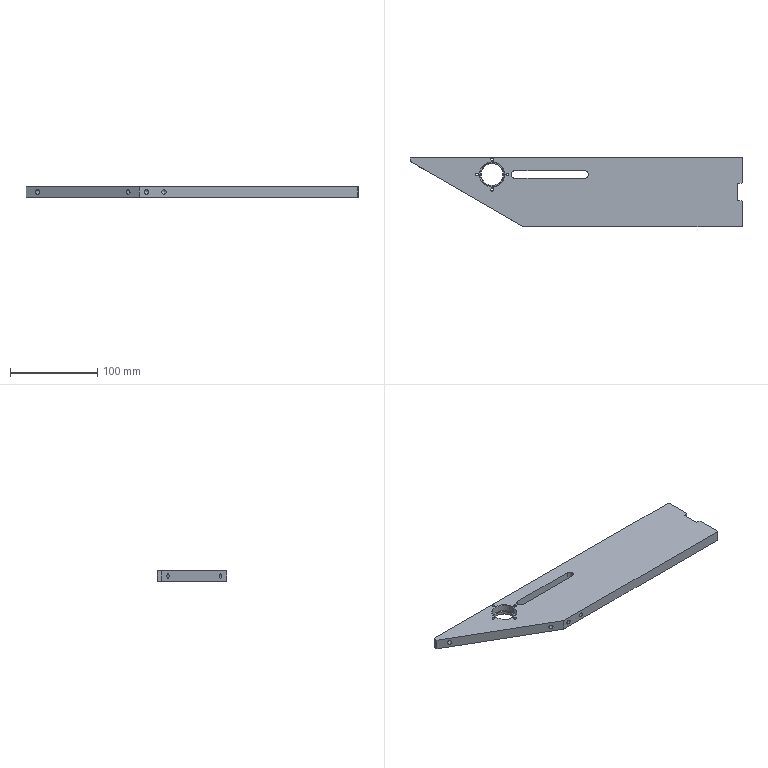Part | NX | 1 solid | 42 faces | box 380 x 80 x 12 mm | volume 287140 mm3 | plane 19 | cylinder 14 | cone 9 | commonest cylinder face diameters 5 x6 3.3 x4 8.5 x2 25 x1 28 x1
STEP:
#1=CARTESIAN_POINT('',(190.,-32.5,-6.));
#2=VERTEX_POINT('',#1);
#3=CARTESIAN_POINT('',(190.,-30.,-6.));
#4=DIRECTION('',(1.,0.,0.));
#5=DIRECTION('',(0.,-1.,0.));
#6=AXIS2_PLACEMENT_3D('',#3,#4,#5);
#7=CIRCLE('',#6,2.5);
#8=EDGE_CURVE('',#2,#2,#7,.T.);
#9=ORIENTED_EDGE('',*,*,#8,.F.);
#10=EDGE_LOOP('',(#9));
#11=FACE_BOUND('',#10,.T.);
#12=CARTESIAN_POINT('',(190.,-11.,-12.));
#13=VERTEX_POINT('',#12);
#14=CARTESIAN_POINT('',(190.,-39.,-12.));
#15=VERTEX_POINT('',#14);
#16=CARTESIAN_POINT('',(190.,40.,-12.));
#17=DIRECTION('',(0.,-1.,0.));
#18=VECTOR('',#17,1000.);
#19=LINE('',#16,#18);
#20=EDGE_CURVE('',#13,#15,#19,.T.);
#21=ORIENTED_EDGE('',*,*,#20,.F.);
#22=CARTESIAN_POINT('',(190.,-11.,0.));
#23=VERTEX_POINT('',#22);
#24=CARTESIAN_POINT('',(190.,-11.,-12.));
#25=DIRECTION('',(0.,0.,1.));
#26=VECTOR('',#25,1000.);
#27=LINE('',#24,#26);
#28=EDGE_CURVE('',#13,#23,#27,.T.);
#29=ORIENTED_EDGE('',*,*,#28,.T.);
#30=CARTESIAN_POINT('',(190.,-39.,0.));
#31=VERTEX_POINT('',#30);
#32=CARTESIAN_POINT('',(190.,40.,0.));
#33=DIRECTION('',(0.,-1.,0.));
#34=VECTOR('',#33,1000.);
#35=LINE('',#32,#34);
#36=EDGE_CURVE('',#23,#31,#35,.T.);
#37=ORIENTED_EDGE('',*,*,#36,.T.);
#38=CARTESIAN_POINT('',(190.,-39.,-12.));
#39=DIRECTION('',(0.,0.,-1.));
#40=VECTOR('',#39,1000.);
#41=LINE('',#38,#40);
#42=EDGE_CURVE('',#31,#15,#41,.T.);
#43=ORIENTED_EDGE('',*,*,#42,.T.);
#44=EDGE_LOOP('',(#21,#29,#37,#43));
#45=FACE_BOUND('',#44,.T.);
#46=CARTESIAN_POINT('',(190.,40.,-12.));
#47=DIRECTION('',(-1.,0.,0.));
#48=DIRECTION('',(0.,1.,0.));
#49=AXIS2_PLACEMENT_3D('',#46,#47,#48);
#50=PLANE('',#49);
#51=ADVANCED_FACE('',(#11,#45),#50,.F.);
#52=CARTESIAN_POINT('',(-96.,32.5,-8.5));
#53=VERTEX_POINT('',#52);
#54=CARTESIAN_POINT('',(-96.,20.,-8.5));
#55=DIRECTION('',(0.,0.,1.));
#56=DIRECTION('',(0.,1.,0.));
#57=AXIS2_PLACEMENT_3D('',#54,#55,#56);
#58=CIRCLE('',#57,12.5);
#59=EDGE_CURVE('',#53,#53,#58,.T.);
#60=ORIENTED_EDGE('',*,*,#59,.T.);
#61=EDGE_LOOP('',(#60));
#62=FACE_BOUND('',#61,.T.);
#63=CARTESIAN_POINT('',(-96.,32.5,-11.5));
#64=VERTEX_POINT('',#63);
#65=CARTESIAN_POINT('',(-96.,20.,-11.5));
#66=DIRECTION('',(0.,0.,1.));
#67=DIRECTION('',(0.,1.,0.));
#68=AXIS2_PLACEMENT_3D('',#65,#66,#67);
#69=CIRCLE('',#68,12.5);
#70=EDGE_CURVE('',#64,#64,#69,.F.);
#71=ORIENTED_EDGE('',*,*,#70,.T.);
#72=EDGE_LOOP('',(#71));
#73=FACE_BOUND('',#72,.T.);
#74=CARTESIAN_POINT('',(-96.,20.,0.));
#75=DIRECTION('',(0.,0.,-1.));
#76=DIRECTION('',(0.,-1.,0.));
#77=AXIS2_PLACEMENT_3D('',#74,#75,#76);
#78=CYLINDRICAL_SURFACE('',#77,12.5);
#79=ADVANCED_FACE('',(#62,#73),#78,.F.);
#80=CARTESIAN_POINT('',(-168.66,40.,-8.3));
#81=VERTEX_POINT('',#80);
#82=CARTESIAN_POINT('',(-168.66,40.,-3.7));
#83=VERTEX_POINT('',#82);
#84=CARTESIAN_POINT('',(-168.66,40.,-8.3));
#85=CARTESIAN_POINT('',(-168.16,40.,-7.644));
#86=CARTESIAN_POINT('',(-167.409,40.,-6.001));
#87=CARTESIAN_POINT('',(-168.153,40.,-4.365));
#88=CARTESIAN_POINT('',(-168.66,40.,-3.7));
#89=B_SPLINE_CURVE_WITH_KNOTS('',3,(#84,#85,#86,#87,#88),.UNSPECIFIED.,.F.,.F.,(4,1,4),(0.001159,0.003632,0.006106),.UNSPECIFIED.);
#90=EDGE_CURVE('',#81,#83,#89,.T.);
#91=ORIENTED_EDGE('',*,*,#90,.T.);
#92=CARTESIAN_POINT('',(-169.793,40.,-6.));
#93=DIRECTION('',(0.,-1.,0.));
#94=DIRECTION('',(-1.,0.,0.));
#95=AXIS2_PLACEMENT_3D('',#92,#93,#94);
#96=ELLIPSE('',#95,2.887,2.5);
#97=EDGE_CURVE('',#83,#81,#96,.T.);
#98=ORIENTED_EDGE('',*,*,#97,.T.);
#99=EDGE_LOOP('',(#91,#98));
#100=FACE_BOUND('',#99,.T.);
#101=CARTESIAN_POINT('',(-189.,40.,-12.));
#102=VERTEX_POINT('',#101);
#103=CARTESIAN_POINT('',(189.,40.,-12.));
#104=VERTEX_POINT('',#103);
#105=CARTESIAN_POINT('',(190.,40.,-12.));
#106=DIRECTION('',(1.,0.,0.));
#107=VECTOR('',#106,1000.);
#108=LINE('',#105,#107);
#109=EDGE_CURVE('',#102,#104,#108,.T.);
#110=ORIENTED_EDGE('',*,*,#109,.F.);
#111=CARTESIAN_POINT('',(-189.,40.,0.));
#112=VERTEX_POINT('',#111);
#113=CARTESIAN_POINT('',(-189.,40.,-12.));
#114=DIRECTION('',(0.,0.,1.));
#115=VECTOR('',#114,1000.);
#116=LINE('',#113,#115);
#117=EDGE_CURVE('',#102,#112,#116,.T.);
#118=ORIENTED_EDGE('',*,*,#117,.T.);
#119=CARTESIAN_POINT('',(189.,40.,0.));
#120=VERTEX_POINT('',#119);
#121=CARTESIAN_POINT('',(190.,40.,0.));
#122=DIRECTION('',(1.,0.,0.));
#123=VECTOR('',#122,1000.);
#124=LINE('',#121,#123);
#125=EDGE_CURVE('',#112,#120,#124,.T.);
#126=ORIENTED_EDGE('',*,*,#125,.T.);
#127=CARTESIAN_POINT('',(189.,40.,-12.));
#128=DIRECTION('',(0.,0.,-1.));
#129=VECTOR('',#128,1000.);
#130=LINE('',#127,#129);
#131=EDGE_CURVE('',#120,#104,#130,.T.);
#132=ORIENTED_EDGE('',*,*,#131,.T.);
#133=EDGE_LOOP('',(#110,#118,#126,#132));
#134=FACE_BOUND('',#133,.T.);
#135=CARTESIAN_POINT('',(190.,40.,-12.));
#136=DIRECTION('',(0.,-1.,0.));
#137=DIRECTION('',(0.,0.,1.));
#138=AXIS2_PLACEMENT_3D('',#135,#136,#137);
#139=PLANE('',#138);
#140=ADVANCED_FACE('',(#100,#134),#139,.F.);
#141=CARTESIAN_POINT('',(190.,27.5,-6.));
#142=VERTEX_POINT('',#141);
#143=CARTESIAN_POINT('',(190.,30.,-6.));
#144=DIRECTION('',(1.,0.,0.));
#145=DIRECTION('',(0.,-1.,0.));
#146=AXIS2_PLACEMENT_3D('',#143,#144,#145);
#147=CIRCLE('',#146,2.5);
#148=EDGE_CURVE('',#142,#142,#147,.T.);
#149=ORIENTED_EDGE('',*,*,#148,.F.);
#150=EDGE_LOOP('',(#149));
#151=FACE_BOUND('',#150,.T.);
#152=CARTESIAN_POINT('',(190.,39.,0.));
#153=VERTEX_POINT('',#152);
#154=CARTESIAN_POINT('',(190.,11.,0.));
#155=VERTEX_POINT('',#154);
#156=CARTESIAN_POINT('',(190.,40.,0.));
#157=DIRECTION('',(0.,-1.,0.));
#158=VECTOR('',#157,1000.);
#159=LINE('',#156,#158);
#160=EDGE_CURVE('',#153,#155,#159,.T.);
#161=ORIENTED_EDGE('',*,*,#160,.T.);
#162=CARTESIAN_POINT('',(190.,11.,-12.));
#163=VERTEX_POINT('',#162);
#164=CARTESIAN_POINT('',(190.,11.,-12.));
#165=DIRECTION('',(0.,0.,-1.));
#166=VECTOR('',#165,1000.);
#167=LINE('',#164,#166);
#168=EDGE_CURVE('',#155,#163,#167,.T.);
#169=ORIENTED_EDGE('',*,*,#168,.T.);
#170=CARTESIAN_POINT('',(190.,39.,-12.));
#171=VERTEX_POINT('',#170);
#172=CARTESIAN_POINT('',(190.,40.,-12.));
#173=DIRECTION('',(0.,-1.,0.));
#174=VECTOR('',#173,1000.);
#175=LINE('',#172,#174);
#176=EDGE_CURVE('',#171,#163,#175,.T.);
#177=ORIENTED_EDGE('',*,*,#176,.F.);
#178=CARTESIAN_POINT('',(190.,39.,-12.));
#179=DIRECTION('',(0.,0.,1.));
#180=VECTOR('',#179,1000.);
#181=LINE('',#178,#180);
#182=EDGE_CURVE('',#171,#153,#181,.T.);
#183=ORIENTED_EDGE('',*,*,#182,.T.);
#184=EDGE_LOOP('',(#161,#169,#177,#183));
#185=FACE_BOUND('',#184,.T.);
#186=CARTESIAN_POINT('',(190.,40.,-12.));
#187=DIRECTION('',(-1.,0.,0.));
#188=DIRECTION('',(0.,1.,0.));
#189=AXIS2_PLACEMENT_3D('',#186,#187,#188);
#190=PLANE('',#189);
#191=ADVANCED_FACE('',(#151,#185),#190,.F.);
#192=CARTESIAN_POINT('',(-52.096,-40.,-3.5));
#193=VERTEX_POINT('',#192);
#194=CARTESIAN_POINT('',(-52.096,-40.,-6.));
#195=DIRECTION('',(0.,-1.,0.));
#196=DIRECTION('',(0.,0.,1.));
#197=AXIS2_PLACEMENT_3D('',#194,#195,#196);
#198=CIRCLE('',#197,2.5);
#199=EDGE_CURVE('',#193,#193,#198,.T.);
#200=ORIENTED_EDGE('',*,*,#199,.F.);
#201=EDGE_LOOP('',(#200));
#202=FACE_BOUND('',#201,.T.);
#203=CARTESIAN_POINT('',(-32.096,-40.,-3.5));
#204=VERTEX_POINT('',#203);
#205=CARTESIAN_POINT('',(-32.096,-40.,-6.));
#206=DIRECTION('',(0.,-1.,0.));
#207=DIRECTION('',(0.,0.,1.));
#208=AXIS2_PLACEMENT_3D('',#205,#206,#207);
#209=CIRCLE('',#208,2.5);
#210=EDGE_CURVE('',#204,#204,#209,.T.);
#211=ORIENTED_EDGE('',*,*,#210,.F.);
#212=EDGE_LOOP('',(#211));
#213=FACE_BOUND('',#212,.T.);
#214=CARTESIAN_POINT('',(189.,-40.,-12.));
#215=VERTEX_POINT('',#214);
#216=CARTESIAN_POINT('',(-60.096,-40.,-12.));
#217=VERTEX_POINT('',#216);
#218=CARTESIAN_POINT('',(190.,-40.,-12.));
#219=DIRECTION('',(-1.,0.,0.));
#220=VECTOR('',#219,1000.);
#221=LINE('',#218,#220);
#222=EDGE_CURVE('',#215,#217,#221,.T.);
#223=ORIENTED_EDGE('',*,*,#222,.F.);
#224=CARTESIAN_POINT('',(189.,-40.,0.));
#225=VERTEX_POINT('',#224);
#226=CARTESIAN_POINT('',(189.,-40.,-12.));
#227=DIRECTION('',(0.,0.,1.));
#228=VECTOR('',#227,1000.);
#229=LINE('',#226,#228);
#230=EDGE_CURVE('',#215,#225,#229,.T.);
#231=ORIENTED_EDGE('',*,*,#230,.T.);
#232=CARTESIAN_POINT('',(-60.096,-40.,0.));
#233=VERTEX_POINT('',#232);
#234=CARTESIAN_POINT('',(190.,-40.,0.));
#235=DIRECTION('',(-1.,0.,0.));
#236=VECTOR('',#235,1000.);
#237=LINE('',#234,#236);
#238=EDGE_CURVE('',#225,#233,#237,.T.);
#239=ORIENTED_EDGE('',*,*,#238,.T.);
#240=CARTESIAN_POINT('',(-60.096,-40.,-12.));
#241=DIRECTION('',(0.,0.,1.));
#242=VECTOR('',#241,1000.);
#243=LINE('',#240,#242);
#244=EDGE_CURVE('',#217,#233,#243,.T.);
#245=ORIENTED_EDGE('',*,*,#244,.F.);
#246=EDGE_LOOP('',(#223,#231,#239,#245));
#247=FACE_BOUND('',#246,.T.);
#248=CARTESIAN_POINT('',(190.,-40.,-12.));
#249=DIRECTION('',(0.,1.,0.));
#250=DIRECTION('',(0.,0.,-1.));
#251=AXIS2_PLACEMENT_3D('',#248,#249,#250);
#252=PLANE('',#251);
#253=ADVANCED_FACE('',(#202,#213,#247),#252,.F.);
#254=CARTESIAN_POINT('',(-179.175,28.75,-6.));
#255=VERTEX_POINT('',#254);
#256=CARTESIAN_POINT('',(-177.01,27.5,-6.));
#257=DIRECTION('',(-0.5,-0.866,0.));
#258=DIRECTION('',(-0.866,0.5,0.));
#259=AXIS2_PLACEMENT_3D('',#256,#257,#258);
#260=CIRCLE('',#259,2.5);
#261=EDGE_CURVE('',#255,#255,#260,.T.);
#262=ORIENTED_EDGE('',*,*,#261,.F.);
#263=EDGE_LOOP('',(#262));
#264=FACE_BOUND('',#263,.T.);
#265=CARTESIAN_POINT('',(-75.252,-31.25,-6.));
#266=VERTEX_POINT('',#265);
#267=CARTESIAN_POINT('',(-73.087,-32.5,-6.));
#268=DIRECTION('',(-0.5,-0.866,0.));
#269=DIRECTION('',(-0.866,0.5,0.));
#270=AXIS2_PLACEMENT_3D('',#267,#268,#269);
#271=CIRCLE('',#270,2.5);
#272=EDGE_CURVE('',#266,#266,#271,.T.);
#273=ORIENTED_EDGE('',*,*,#272,.F.);
#274=EDGE_LOOP('',(#273));
#275=FACE_BOUND('',#274,.T.);
#276=CARTESIAN_POINT('',(-190.,35.,0.));
#277=VERTEX_POINT('',#276);
#278=CARTESIAN_POINT('',(-190.,35.,0.));
#279=DIRECTION('',(-0.866,0.5,0.));
#280=VECTOR('',#279,1000.);
#281=LINE('',#278,#280);
#282=EDGE_CURVE('',#233,#277,#281,.T.);
#283=ORIENTED_EDGE('',*,*,#282,.T.);
#284=CARTESIAN_POINT('',(-190.,35.,-12.));
#285=VERTEX_POINT('',#284);
#286=CARTESIAN_POINT('',(-190.,35.,-12.));
#287=DIRECTION('',(0.,0.,1.));
#288=VECTOR('',#287,1000.);
#289=LINE('',#286,#288);
#290=EDGE_CURVE('',#285,#277,#289,.T.);
#291=ORIENTED_EDGE('',*,*,#290,.F.);
#292=CARTESIAN_POINT('',(-190.,35.,-12.));
#293=DIRECTION('',(-0.866,0.5,0.));
#294=VECTOR('',#293,1000.);
#295=LINE('',#292,#294);
#296=EDGE_CURVE('',#217,#285,#295,.T.);
#297=ORIENTED_EDGE('',*,*,#296,.F.);
#298=ORIENTED_EDGE('',*,*,#244,.T.);
#299=EDGE_LOOP('',(#283,#291,#297,#298));
#300=FACE_BOUND('',#299,.T.);
#301=CARTESIAN_POINT('',(-190.,35.,-12.));
#302=DIRECTION('',(0.5,0.866,0.));
#303=DIRECTION('',(0.866,-0.5,0.));
#304=AXIS2_PLACEMENT_3D('',#301,#302,#303);
#305=PLANE('',#304);
#306=ADVANCED_FACE('',(#264,#275,#300),#305,.F.);
#307=CARTESIAN_POINT('',(-190.,39.,0.));
#308=VERTEX_POINT('',#307);
#309=CARTESIAN_POINT('',(-190.,40.,0.));
#310=DIRECTION('',(0.,1.,0.));
#311=VECTOR('',#310,1000.);
#312=LINE('',#309,#311);
#313=EDGE_CURVE('',#277,#308,#312,.T.);
#314=ORIENTED_EDGE('',*,*,#313,.T.);
#315=CARTESIAN_POINT('',(-190.,39.,-12.));
#316=VERTEX_POINT('',#315);
#317=CARTESIAN_POINT('',(-190.,39.,-12.));
#318=DIRECTION('',(0.,0.,-1.));
#319=VECTOR('',#318,1000.);
#320=LINE('',#317,#319);
#321=EDGE_CURVE('',#308,#316,#320,.T.);
#322=ORIENTED_EDGE('',*,*,#321,.T.);
#323=CARTESIAN_POINT('',(-190.,40.,-12.));
#324=DIRECTION('',(0.,1.,0.));
#325=VECTOR('',#324,1000.);
#326=LINE('',#323,#325);
#327=EDGE_CURVE('',#285,#316,#326,.T.);
#328=ORIENTED_EDGE('',*,*,#327,.F.);
#329=ORIENTED_EDGE('',*,*,#290,.T.);
#330=EDGE_LOOP('',(#314,#322,#328,#329));
#331=FACE_BOUND('',#330,.T.);
#332=CARTESIAN_POINT('',(-190.,40.,-12.));
#333=DIRECTION('',(1.,0.,0.));
#334=DIRECTION('',(0.,-1.,0.));
#335=AXIS2_PLACEMENT_3D('',#332,#333,#334);
#336=PLANE('',#335);
#337=ADVANCED_FACE('',(#331),#336,.F.);
#338=CARTESIAN_POINT('',(10.,24.25,-12.));
#339=VERTEX_POINT('',#338);
#340=CARTESIAN_POINT('',(-70.,24.25,-12.));
#341=VERTEX_POINT('',#340);
#342=CARTESIAN_POINT('',(-70.,24.25,-12.));
#343=DIRECTION('',(-1.,0.,0.));
#344=VECTOR('',#343,1000.);
#345=LINE('',#342,#344);
#346=EDGE_CURVE('',#339,#341,#345,.T.);
#347=ORIENTED_EDGE('',*,*,#346,.T.);
#348=CARTESIAN_POINT('',(-70.,15.75,-12.));
#349=VERTEX_POINT('',#348);
#350=CARTESIAN_POINT('',(-70.,20.,-12.));
#351=DIRECTION('',(0.,0.,1.));
#352=DIRECTION('',(0.,1.,0.));
#353=AXIS2_PLACEMENT_3D('',#350,#351,#352);
#354=CIRCLE('',#353,4.25);
#355=EDGE_CURVE('',#341,#349,#354,.T.);
#356=ORIENTED_EDGE('',*,*,#355,.T.);
#357=CARTESIAN_POINT('',(10.,15.75,-12.));
#358=VERTEX_POINT('',#357);
#359=CARTESIAN_POINT('',(-70.,15.75,-12.));
#360=DIRECTION('',(1.,0.,0.));
#361=VECTOR('',#360,1000.);
#362=LINE('',#359,#361);
#363=EDGE_CURVE('',#349,#358,#362,.T.);
#364=ORIENTED_EDGE('',*,*,#363,.T.);
#365=CARTESIAN_POINT('',(10.,20.,-12.));
#366=DIRECTION('',(0.,0.,1.));
#367=DIRECTION('',(0.,1.,0.));
#368=AXIS2_PLACEMENT_3D('',#365,#366,#367);
#369=CIRCLE('',#368,4.25);
#370=EDGE_CURVE('',#358,#339,#369,.T.);
#371=ORIENTED_EDGE('',*,*,#370,.T.);
#372=EDGE_LOOP('',(#347,#356,#364,#371));
#373=FACE_BOUND('',#372,.T.);
#374=CARTESIAN_POINT('',(-96.,33.,-12.));
#375=VERTEX_POINT('',#374);
#376=CARTESIAN_POINT('',(-96.,20.,-12.));
#377=DIRECTION('',(0.,0.,1.));
#378=DIRECTION('',(0.,1.,0.));
#379=AXIS2_PLACEMENT_3D('',#376,#377,#378);
#380=CIRCLE('',#379,13.);
#381=EDGE_CURVE('',#375,#375,#380,.T.);
#382=ORIENTED_EDGE('',*,*,#381,.T.);
#383=EDGE_LOOP('',(#382));
#384=FACE_BOUND('',#383,.T.);
#385=CARTESIAN_POINT('',(-94.35,37.5,-12.));
#386=VERTEX_POINT('',#385);
#387=CARTESIAN_POINT('',(-96.,37.5,-12.));
#388=DIRECTION('',(0.,0.,1.));
#389=DIRECTION('',(1.,0.,0.));
#390=AXIS2_PLACEMENT_3D('',#387,#388,#389);
#391=CIRCLE('',#390,1.65);
#392=EDGE_CURVE('',#386,#386,#391,.T.);
#393=ORIENTED_EDGE('',*,*,#392,.T.);
#394=EDGE_LOOP('',(#393));
#395=FACE_BOUND('',#394,.T.);
#396=CARTESIAN_POINT('',(-78.5,18.35,-12.));
#397=VERTEX_POINT('',#396);
#398=CARTESIAN_POINT('',(-78.5,20.,-12.));
#399=DIRECTION('',(0.,0.,1.));
#400=DIRECTION('',(0.,-1.,0.));
#401=AXIS2_PLACEMENT_3D('',#398,#399,#400);
#402=CIRCLE('',#401,1.65);
#403=EDGE_CURVE('',#397,#397,#402,.T.);
#404=ORIENTED_EDGE('',*,*,#403,.T.);
#405=EDGE_LOOP('',(#404));
#406=FACE_BOUND('',#405,.T.);
#407=CARTESIAN_POINT('',(-97.65,2.5,-12.));
#408=VERTEX_POINT('',#407);
#409=CARTESIAN_POINT('',(-96.,2.5,-12.));
#410=DIRECTION('',(0.,0.,1.));
#411=DIRECTION('',(-1.,0.,0.));
#412=AXIS2_PLACEMENT_3D('',#409,#410,#411);
#413=CIRCLE('',#412,1.65);
#414=EDGE_CURVE('',#408,#408,#413,.T.);
#415=ORIENTED_EDGE('',*,*,#414,.T.);
#416=EDGE_LOOP('',(#415));
#417=FACE_BOUND('',#416,.T.);
#418=CARTESIAN_POINT('',(-113.5,21.65,-12.));
#419=VERTEX_POINT('',#418);
#420=CARTESIAN_POINT('',(-113.5,20.,-12.));
#421=DIRECTION('',(0.,0.,1.));
#422=DIRECTION('',(0.,1.,0.));
#423=AXIS2_PLACEMENT_3D('',#420,#421,#422);
#424=CIRCLE('',#423,1.65);
#425=EDGE_CURVE('',#419,#419,#424,.T.);
#426=ORIENTED_EDGE('',*,*,#425,.T.);
#427=EDGE_LOOP('',(#426));
#428=FACE_BOUND('',#427,.T.);
#429=CARTESIAN_POINT('',(189.,-10.,-12.));
#430=VERTEX_POINT('',#429);
#431=CARTESIAN_POINT('',(185.,-10.,-12.));
#432=VERTEX_POINT('',#431);
#433=CARTESIAN_POINT('',(195.,-10.,-12.));
#434=DIRECTION('',(-1.,0.,0.));
#435=VECTOR('',#434,1000.);
#436=LINE('',#433,#435);
#437=EDGE_CURVE('',#430,#432,#436,.T.);
#438=ORIENTED_EDGE('',*,*,#437,.F.);
#439=CARTESIAN_POINT('',(190.,-11.,-12.));
#440=DIRECTION('',(-0.7071,0.7071,0.));
#441=VECTOR('',#440,1000.);
#442=LINE('',#439,#441);
#443=EDGE_CURVE('',#430,#13,#442,.F.);
#444=ORIENTED_EDGE('',*,*,#443,.T.);
#445=ORIENTED_EDGE('',*,*,#20,.T.);
#446=CARTESIAN_POINT('',(189.,-40.,-12.));
#447=DIRECTION('',(0.7071,0.7071,0.));
#448=VECTOR('',#447,1000.);
#449=LINE('',#446,#448);
#450=EDGE_CURVE('',#15,#215,#449,.F.);
#451=ORIENTED_EDGE('',*,*,#450,.T.);
#452=ORIENTED_EDGE('',*,*,#222,.T.);
#453=ORIENTED_EDGE('',*,*,#296,.T.);
#454=ORIENTED_EDGE('',*,*,#327,.T.);
#455=CARTESIAN_POINT('',(-189.,40.,-12.));
#456=DIRECTION('',(-0.7071,-0.7071,0.));
#457=VECTOR('',#456,1000.);
#458=LINE('',#455,#457);
#459=EDGE_CURVE('',#316,#102,#458,.F.);
#460=ORIENTED_EDGE('',*,*,#459,.T.);
#461=ORIENTED_EDGE('',*,*,#109,.T.);
#462=CARTESIAN_POINT('',(190.,39.,-12.));
#463=DIRECTION('',(-0.7071,0.7071,0.));
#464=VECTOR('',#463,1000.);
#465=LINE('',#462,#464);
#466=EDGE_CURVE('',#104,#171,#465,.F.);
#467=ORIENTED_EDGE('',*,*,#466,.T.);
#468=ORIENTED_EDGE('',*,*,#176,.T.);
#469=CARTESIAN_POINT('',(189.,10.,-12.));
#470=VERTEX_POINT('',#469);
#471=CARTESIAN_POINT('',(190.,11.,-12.));
#472=DIRECTION('',(0.7071,0.7071,0.));
#473=VECTOR('',#472,1000.);
#474=LINE('',#471,#473);
#475=EDGE_CURVE('',#163,#470,#474,.F.);
#476=ORIENTED_EDGE('',*,*,#475,.T.);
#477=CARTESIAN_POINT('',(185.,10.,-12.));
#478=VERTEX_POINT('',#477);
#479=CARTESIAN_POINT('',(195.,10.,-12.));
#480=DIRECTION('',(1.,0.,0.));
#481=VECTOR('',#480,1000.);
#482=LINE('',#479,#481);
#483=EDGE_CURVE('',#478,#470,#482,.T.);
#484=ORIENTED_EDGE('',*,*,#483,.F.);
#485=CARTESIAN_POINT('',(185.,10.,-12.));
#486=DIRECTION('',(0.,1.,0.));
#487=VECTOR('',#486,1000.);
#488=LINE('',#485,#487);
#489=EDGE_CURVE('',#432,#478,#488,.T.);
#490=ORIENTED_EDGE('',*,*,#489,.F.);
#491=EDGE_LOOP('',(#438,#444,#445,#451,#452,#453,#454,#460,#461,#467,#468,#476,#484,#490));
#492=FACE_BOUND('',#491,.T.);
#493=CARTESIAN_POINT('',(190.,40.,-12.));
#494=DIRECTION('',(0.,0.,1.));
#495=DIRECTION('',(0.,1.,0.));
#496=AXIS2_PLACEMENT_3D('',#493,#494,#495);
#497=PLANE('',#496);
#498=ADVANCED_FACE('',(#373,#384,#395,#406,#417,#428,#492),#497,.F.);
#499=CARTESIAN_POINT('',(-70.,24.25,0.));
#500=VERTEX_POINT('',#499);
#501=CARTESIAN_POINT('',(-70.,15.75,0.));
#502=VERTEX_POINT('',#501);
#503=CARTESIAN_POINT('',(-70.,20.,0.));
#504=DIRECTION('',(0.,0.,1.));
#505=DIRECTION('',(0.,1.,0.));
#506=AXIS2_PLACEMENT_3D('',#503,#504,#505);
#507=CIRCLE('',#506,4.25);
#508=EDGE_CURVE('',#500,#502,#507,.T.);
#509=ORIENTED_EDGE('',*,*,#508,.F.);
#510=CARTESIAN_POINT('',(10.,24.25,0.));
#511=VERTEX_POINT('',#510);
#512=CARTESIAN_POINT('',(-70.,24.25,0.));
#513=DIRECTION('',(-1.,0.,0.));
#514=VECTOR('',#513,1000.);
#515=LINE('',#512,#514);
#516=EDGE_CURVE('',#511,#500,#515,.T.);
#517=ORIENTED_EDGE('',*,*,#516,.F.);
#518=CARTESIAN_POINT('',(10.,15.75,0.));
#519=VERTEX_POINT('',#518);
#520=CARTESIAN_POINT('',(10.,20.,0.));
#521=DIRECTION('',(0.,0.,1.));
#522=DIRECTION('',(0.,1.,0.));
#523=AXIS2_PLACEMENT_3D('',#520,#521,#522);
#524=CIRCLE('',#523,4.25);
#525=EDGE_CURVE('',#519,#511,#524,.T.);
#526=ORIENTED_EDGE('',*,*,#525,.F.);
#527=CARTESIAN_POINT('',(-70.,15.75,0.));
#528=DIRECTION('',(1.,0.,0.));
#529=VECTOR('',#528,1000.);
#530=LINE('',#527,#529);
#531=EDGE_CURVE('',#502,#519,#530,.T.);
#532=ORIENTED_EDGE('',*,*,#531,.F.);
#533=EDGE_LOOP('',(#509,#517,#526,#532));
#534=FACE_BOUND('',#533,.T.);
#535=ORIENTED_EDGE('',*,*,#36,.F.);
#536=CARTESIAN_POINT('',(189.,-10.,0.));
#537=VERTEX_POINT('',#536);
#538=CARTESIAN_POINT('',(164.5,14.5,0.));
#539=DIRECTION('',(0.7071,-0.7071,0.));
#540=VECTOR('',#539,1000.);
#541=LINE('',#538,#540);
#542=EDGE_CURVE('',#23,#537,#541,.F.);
#543=ORIENTED_EDGE('',*,*,#542,.T.);
#544=CARTESIAN_POINT('',(185.,-10.,0.));
#545=VERTEX_POINT('',#544);
#546=CARTESIAN_POINT('',(190.,-10.,0.));
#547=DIRECTION('',(1.,0.,0.));
#548=VECTOR('',#547,1000.);
#549=LINE('',#546,#548);
#550=EDGE_CURVE('',#545,#537,#549,.T.);
#551=ORIENTED_EDGE('',*,*,#550,.F.);
#552=CARTESIAN_POINT('',(185.,10.,0.));
#553=VERTEX_POINT('',#552);
#554=CARTESIAN_POINT('',(185.,10.,0.));
#555=DIRECTION('',(0.,1.,0.));
#556=VECTOR('',#555,1000.);
#557=LINE('',#554,#556);
#558=EDGE_CURVE('',#545,#553,#557,.T.);
#559=ORIENTED_EDGE('',*,*,#558,.T.);
#560=CARTESIAN_POINT('',(189.,10.,0.));
#561=VERTEX_POINT('',#560);
#562=CARTESIAN_POINT('',(195.,10.,0.));
#563=DIRECTION('',(1.,0.,0.));
#564=VECTOR('',#563,1000.);
#565=LINE('',#562,#564);
#566=EDGE_CURVE('',#553,#561,#565,.T.);
#567=ORIENTED_EDGE('',*,*,#566,.T.);
#568=CARTESIAN_POINT('',(204.5,25.5,0.));
#569=DIRECTION('',(-0.7071,-0.7071,0.));
#570=VECTOR('',#569,1000.);
#571=LINE('',#568,#570);
#572=EDGE_CURVE('',#561,#155,#571,.F.);
#573=ORIENTED_EDGE('',*,*,#572,.T.);
#574=ORIENTED_EDGE('',*,*,#160,.F.);
#575=CARTESIAN_POINT('',(189.5,39.5,0.));
#576=DIRECTION('',(0.7071,-0.7071,0.));
#577=VECTOR('',#576,1000.);
#578=LINE('',#575,#577);
#579=EDGE_CURVE('',#153,#120,#578,.F.);
#580=ORIENTED_EDGE('',*,*,#579,.T.);
#581=ORIENTED_EDGE('',*,*,#125,.F.);
#582=CARTESIAN_POINT('',(0.5,229.5,0.));
#583=DIRECTION('',(0.7071,0.7071,0.));
#584=VECTOR('',#583,1000.);
#585=LINE('',#582,#584);
#586=EDGE_CURVE('',#112,#308,#585,.F.);
#587=ORIENTED_EDGE('',*,*,#586,.T.);
#588=ORIENTED_EDGE('',*,*,#313,.F.);
#589=ORIENTED_EDGE('',*,*,#282,.F.);
#590=ORIENTED_EDGE('',*,*,#238,.F.);
#591=CARTESIAN_POINT('',(229.5,0.5,0.));
#592=DIRECTION('',(-0.7071,-0.7071,0.));
#593=VECTOR('',#592,1000.);
#594=LINE('',#591,#593);
#595=EDGE_CURVE('',#225,#31,#594,.F.);
#596=ORIENTED_EDGE('',*,*,#595,.T.);
#597=EDGE_LOOP('',(#535,#543,#551,#559,#567,#573,#574,#580,#581,#587,#588,#589,#590,#596));
#598=FACE_BOUND('',#597,.T.);
#599=CARTESIAN_POINT('',(-96.,34.5,0.));
#600=VERTEX_POINT('',#599);
#601=CARTESIAN_POINT('',(-96.,20.,0.));
#602=DIRECTION('',(0.,0.,1.));
#603=DIRECTION('',(0.,1.,0.));
#604=AXIS2_PLACEMENT_3D('',#601,#602,#603);
#605=CIRCLE('',#604,14.5);
#606=EDGE_CURVE('',#600,#600,#605,.F.);
#607=ORIENTED_EDGE('',*,*,#606,.T.);
#608=EDGE_LOOP('',(#607));
#609=FACE_BOUND('',#608,.T.);
#610=CARTESIAN_POINT('',(-94.35,37.5,0.));
#611=VERTEX_POINT('',#610);
#612=CARTESIAN_POINT('',(-96.,37.5,0.));
#613=DIRECTION('',(0.,0.,1.));
#614=DIRECTION('',(1.,0.,0.));
#615=AXIS2_PLACEMENT_3D('',#612,#613,#614);
#616=CIRCLE('',#615,1.65);
#617=EDGE_CURVE('',#611,#611,#616,.T.);
#618=ORIENTED_EDGE('',*,*,#617,.F.);
#619=EDGE_LOOP('',(#618));
#620=FACE_BOUND('',#619,.T.);
#621=CARTESIAN_POINT('',(-78.5,18.35,0.));
#622=VERTEX_POINT('',#621);
#623=CARTESIAN_POINT('',(-78.5,20.,0.));
#624=DIRECTION('',(0.,0.,1.));
#625=DIRECTION('',(0.,-1.,0.));
#626=AXIS2_PLACEMENT_3D('',#623,#624,#625);
#627=CIRCLE('',#626,1.65);
#628=EDGE_CURVE('',#622,#622,#627,.T.);
#629=ORIENTED_EDGE('',*,*,#628,.F.);
#630=EDGE_LOOP('',(#629));
#631=FACE_BOUND('',#630,.T.);
#632=CARTESIAN_POINT('',(-97.65,2.5,0.));
#633=VERTEX_POINT('',#632);
#634=CARTESIAN_POINT('',(-96.,2.5,0.));
#635=DIRECTION('',(0.,0.,1.));
#636=DIRECTION('',(-1.,0.,0.));
#637=AXIS2_PLACEMENT_3D('',#634,#635,#636);
#638=CIRCLE('',#637,1.65);
#639=EDGE_CURVE('',#633,#633,#638,.T.);
#640=ORIENTED_EDGE('',*,*,#639,.F.);
#641=EDGE_LOOP('',(#640));
#642=FACE_BOUND('',#641,.T.);
#643=CARTESIAN_POINT('',(-113.5,21.65,0.));
#644=VERTEX_POINT('',#643);
#645=CARTESIAN_POINT('',(-113.5,20.,0.));
#646=DIRECTION('',(0.,0.,1.));
#647=DIRECTION('',(0.,1.,0.));
#648=AXIS2_PLACEMENT_3D('',#645,#646,#647);
#649=CIRCLE('',#648,1.65);
#650=EDGE_CURVE('',#644,#644,#649,.T.);
#651=ORIENTED_EDGE('',*,*,#650,.F.);
#652=EDGE_LOOP('',(#651));
#653=FACE_BOUND('',#652,.T.);
#654=CARTESIAN_POINT('',(190.,40.,0.));
#655=DIRECTION('',(0.,0.,1.));
#656=DIRECTION('',(0.,1.,0.));
#657=AXIS2_PLACEMENT_3D('',#654,#655,#656);
#658=PLANE('',#657);
#659=ADVANCED_FACE('',(#534,#598,#609,#620,#631,#642,#653),#658,.T.);
#660=CARTESIAN_POINT('',(-64.865,-18.26,-6.));
#661=VERTEX_POINT('',#660);
#662=VERTEX_LOOP('',#661);
#663=FACE_BOUND('',#662,.T.);
#664=CARTESIAN_POINT('',(-67.752,-18.26,-6.));
#665=VERTEX_POINT('',#664);
#666=CARTESIAN_POINT('',(-65.587,-19.51,-6.));
#667=DIRECTION('',(-0.5,-0.866,0.));
#668=DIRECTION('',(-0.866,0.5,0.));
#669=AXIS2_PLACEMENT_3D('',#666,#667,#668);
#670=CIRCLE('',#669,2.5);
#671=EDGE_CURVE('',#665,#665,#670,.T.);
#672=ORIENTED_EDGE('',*,*,#671,.T.);
#673=EDGE_LOOP('',(#672));
#674=FACE_BOUND('',#673,.T.);
#675=CARTESIAN_POINT('',(-65.587,-19.51,-6.));
#676=DIRECTION('',(-0.5,-0.866,0.));
#677=DIRECTION('',(-0.866,0.5,0.));
#678=AXIS2_PLACEMENT_3D('',#675,#676,#677);
#679=CONICAL_SURFACE('',#678,2.5,1.047);
#680=ADVANCED_FACE('',(#663,#674),#679,.F.);
#681=ORIENTED_EDGE('',*,*,#671,.F.);
#682=EDGE_LOOP('',(#681));
#683=FACE_BOUND('',#682,.T.);
#684=ORIENTED_EDGE('',*,*,#272,.T.);
#685=EDGE_LOOP('',(#684));
#686=FACE_BOUND('',#685,.T.);
#687=CARTESIAN_POINT('',(-73.087,-32.5,-6.));
#688=DIRECTION('',(-0.5,-0.866,0.));
#689=DIRECTION('',(-0.866,0.5,0.));
#690=AXIS2_PLACEMENT_3D('',#687,#688,#689);
#691=CYLINDRICAL_SURFACE('',#690,2.5);
#692=ADVANCED_FACE('',(#683,#686),#691,.F.);
#693=ORIENTED_EDGE('',*,*,#261,.T.);
#694=EDGE_LOOP('',(#693));
#695=FACE_BOUND('',#694,.T.);
#696=CARTESIAN_POINT('',(-169.51,40.49,-6.));
#697=DIRECTION('',(-0.5,-0.866,0.));
#698=DIRECTION('',(-0.866,0.5,0.));
#699=AXIS2_PLACEMENT_3D('',#696,#697,#698);
#700=CIRCLE('',#699,2.5);
#701=EDGE_CURVE('',#81,#83,#700,.T.);
#702=ORIENTED_EDGE('',*,*,#701,.F.);
#703=ORIENTED_EDGE('',*,*,#97,.F.);
#704=EDGE_LOOP('',(#702,#703));
#705=FACE_BOUND('',#704,.T.);
#706=CARTESIAN_POINT('',(-177.01,27.5,-6.));
#707=DIRECTION('',(-0.5,-0.866,0.));
#708=DIRECTION('',(-0.866,0.5,0.));
#709=AXIS2_PLACEMENT_3D('',#706,#707,#708);
#710=CYLINDRICAL_SURFACE('',#709,2.5);
#711=ADVANCED_FACE('',(#695,#705),#710,.F.);
#712=ORIENTED_EDGE('',*,*,#701,.T.);
#713=ORIENTED_EDGE('',*,*,#90,.F.);
#714=EDGE_LOOP('',(#712,#713));
#715=FACE_BOUND('',#714,.T.);
#716=CARTESIAN_POINT('',(-169.51,40.49,-6.));
#717=DIRECTION('',(-0.5,-0.866,0.));
#718=DIRECTION('',(-0.866,0.5,0.));
#719=AXIS2_PLACEMENT_3D('',#716,#717,#718);
#720=CONICAL_SURFACE('',#719,2.5,1.047);
#721=ADVANCED_FACE('',(#715),#720,.F.);
#722=ORIENTED_EDGE('',*,*,#459,.F.);
#723=ORIENTED_EDGE('',*,*,#321,.F.);
#724=ORIENTED_EDGE('',*,*,#586,.F.);
#725=ORIENTED_EDGE('',*,*,#117,.F.);
#726=EDGE_LOOP('',(#722,#723,#724,#725));
#727=FACE_BOUND('',#726,.T.);
#728=CARTESIAN_POINT('',(-189.,40.,-12.));
#729=DIRECTION('',(0.7071,-0.7071,0.));
#730=DIRECTION('',(0.,0.,1.));
#731=AXIS2_PLACEMENT_3D('',#728,#729,#730);
#732=PLANE('',#731);
#733=ADVANCED_FACE('',(#727),#732,.F.);
#734=ORIENTED_EDGE('',*,*,#466,.F.);
#735=ORIENTED_EDGE('',*,*,#131,.F.);
#736=ORIENTED_EDGE('',*,*,#579,.F.);
#737=ORIENTED_EDGE('',*,*,#182,.F.);
#738=EDGE_LOOP('',(#734,#735,#736,#737));
#739=FACE_BOUND('',#738,.T.);
#740=CARTESIAN_POINT('',(190.,39.,-12.));
#741=DIRECTION('',(-0.7071,-0.7071,0.));
#742=DIRECTION('',(0.,0.,1.));
#743=AXIS2_PLACEMENT_3D('',#740,#741,#742);
#744=PLANE('',#743);
#745=ADVANCED_FACE('',(#739),#744,.F.);
#746=ORIENTED_EDGE('',*,*,#450,.F.);
#747=ORIENTED_EDGE('',*,*,#42,.F.);
#748=ORIENTED_EDGE('',*,*,#595,.F.);
#749=ORIENTED_EDGE('',*,*,#230,.F.);
#750=EDGE_LOOP('',(#746,#747,#748,#749));
#751=FACE_BOUND('',#750,.T.);
#752=CARTESIAN_POINT('',(189.,-40.,-12.));
#753=DIRECTION('',(-0.7071,0.7071,0.));
#754=DIRECTION('',(0.,0.,1.));
#755=AXIS2_PLACEMENT_3D('',#752,#753,#754);
#756=PLANE('',#755);
#757=ADVANCED_FACE('',(#751),#756,.F.);
#758=CARTESIAN_POINT('',(-96.,33.,-8.));
#759=VERTEX_POINT('',#758);
#760=CARTESIAN_POINT('',(-96.,20.,-8.));
#761=DIRECTION('',(0.,0.,1.));
#762=DIRECTION('',(0.,1.,0.));
#763=AXIS2_PLACEMENT_3D('',#760,#761,#762);
#764=CIRCLE('',#763,13.);
#765=EDGE_CURVE('',#759,#759,#764,.F.);
#766=ORIENTED_EDGE('',*,*,#765,.T.);
#767=EDGE_LOOP('',(#766));
#768=FACE_BOUND('',#767,.T.);
#769=CARTESIAN_POINT('',(-96.,34.,-8.));
#770=VERTEX_POINT('',#769);
#771=CARTESIAN_POINT('',(-96.,20.,-8.));
#772=DIRECTION('',(0.,0.,1.));
#773=DIRECTION('',(0.,1.,0.));
#774=AXIS2_PLACEMENT_3D('',#771,#772,#773);
#775=CIRCLE('',#774,14.);
#776=EDGE_CURVE('',#770,#770,#775,.T.);
#777=ORIENTED_EDGE('',*,*,#776,.T.);
#778=EDGE_LOOP('',(#777));
#779=FACE_BOUND('',#778,.T.);
#780=CARTESIAN_POINT('',(-96.,20.,-8.));
#781=DIRECTION('',(0.,0.,1.));
#782=DIRECTION('',(0.,1.,0.));
#783=AXIS2_PLACEMENT_3D('',#780,#781,#782);
#784=PLANE('',#783);
#785=ADVANCED_FACE('',(#768,#779),#784,.T.);
#786=CARTESIAN_POINT('',(-96.,34.,-0.5));
#787=VERTEX_POINT('',#786);
#788=CARTESIAN_POINT('',(-96.,20.,-0.5));
#789=DIRECTION('',(0.,0.,1.));
#790=DIRECTION('',(0.,1.,0.));
#791=AXIS2_PLACEMENT_3D('',#788,#789,#790);
#792=CIRCLE('',#791,14.);
#793=EDGE_CURVE('',#787,#787,#792,.T.);
#794=ORIENTED_EDGE('',*,*,#793,.T.);
#795=EDGE_LOOP('',(#794));
#796=FACE_BOUND('',#795,.T.);
#797=ORIENTED_EDGE('',*,*,#776,.F.);
#798=EDGE_LOOP('',(#797));
#799=FACE_BOUND('',#798,.T.);
#800=CARTESIAN_POINT('',(-96.,20.,-8.));
#801=DIRECTION('',(0.,0.,1.));
#802=DIRECTION('',(0.,1.,0.));
#803=AXIS2_PLACEMENT_3D('',#800,#801,#802);
#804=CYLINDRICAL_SURFACE('',#803,14.);
#805=ADVANCED_FACE('',(#796,#799),#804,.F.);
#806=ORIENTED_EDGE('',*,*,#425,.F.);
#807=EDGE_LOOP('',(#806));
#808=FACE_BOUND('',#807,.T.);
#809=ORIENTED_EDGE('',*,*,#650,.T.);
#810=EDGE_LOOP('',(#809));
#811=FACE_BOUND('',#810,.T.);
#812=CARTESIAN_POINT('',(-113.5,20.,0.));
#813=DIRECTION('',(0.,0.,1.));
#814=DIRECTION('',(0.,1.,0.));
#815=AXIS2_PLACEMENT_3D('',#812,#813,#814);
#816=CYLINDRICAL_SURFACE('',#815,1.65);
#817=ADVANCED_FACE('',(#808,#811),#816,.F.);
#818=ORIENTED_EDGE('',*,*,#414,.F.);
#819=EDGE_LOOP('',(#818));
#820=FACE_BOUND('',#819,.T.);
#821=ORIENTED_EDGE('',*,*,#639,.T.);
#822=EDGE_LOOP('',(#821));
#823=FACE_BOUND('',#822,.T.);
#824=CARTESIAN_POINT('',(-96.,2.5,0.));
#825=DIRECTION('',(0.,0.,1.));
#826=DIRECTION('',(-1.,0.,0.));
#827=AXIS2_PLACEMENT_3D('',#824,#825,#826);
#828=CYLINDRICAL_SURFACE('',#827,1.65);
#829=ADVANCED_FACE('',(#820,#823),#828,.F.);
#830=ORIENTED_EDGE('',*,*,#403,.F.);
#831=EDGE_LOOP('',(#830));
#832=FACE_BOUND('',#831,.T.);
#833=ORIENTED_EDGE('',*,*,#628,.T.);
#834=EDGE_LOOP('',(#833));
#835=FACE_BOUND('',#834,.T.);
#836=CARTESIAN_POINT('',(-78.5,20.,0.));
#837=DIRECTION('',(0.,0.,1.));
#838=DIRECTION('',(0.,-1.,0.));
#839=AXIS2_PLACEMENT_3D('',#836,#837,#838);
#840=CYLINDRICAL_SURFACE('',#839,1.65);
#841=ADVANCED_FACE('',(#832,#835),#840,.F.);
#842=ORIENTED_EDGE('',*,*,#392,.F.);
#843=EDGE_LOOP('',(#842));
#844=FACE_BOUND('',#843,.T.);
#845=ORIENTED_EDGE('',*,*,#617,.T.);
#846=EDGE_LOOP('',(#845));
#847=FACE_BOUND('',#846,.T.);
#848=CARTESIAN_POINT('',(-96.,37.5,0.));
#849=DIRECTION('',(0.,0.,1.));
#850=DIRECTION('',(1.,0.,0.));
#851=AXIS2_PLACEMENT_3D('',#848,#849,#850);
#852=CYLINDRICAL_SURFACE('',#851,1.65);
#853=ADVANCED_FACE('',(#844,#847),#852,.F.);
#854=ORIENTED_EDGE('',*,*,#59,.F.);
#855=EDGE_LOOP('',(#854));
#856=FACE_BOUND('',#855,.T.);
#857=ORIENTED_EDGE('',*,*,#765,.F.);
#858=EDGE_LOOP('',(#857));
#859=FACE_BOUND('',#858,.T.);
#860=CARTESIAN_POINT('',(-96.,20.,-8.));
#861=DIRECTION('',(0.,0.,1.));
#862=DIRECTION('',(0.,1.,0.));
#863=AXIS2_PLACEMENT_3D('',#860,#861,#862);
#864=CONICAL_SURFACE('',#863,13.,0.7854);
#865=ADVANCED_FACE('',(#856,#859),#864,.F.);
#866=ORIENTED_EDGE('',*,*,#381,.F.);
#867=EDGE_LOOP('',(#866));
#868=FACE_BOUND('',#867,.T.);
#869=ORIENTED_EDGE('',*,*,#70,.F.);
#870=EDGE_LOOP('',(#869));
#871=FACE_BOUND('',#870,.T.);
#872=CARTESIAN_POINT('',(-96.,20.,-11.5));
#873=DIRECTION('',(0.,0.,-1.));
#874=DIRECTION('',(0.,-1.,0.));
#875=AXIS2_PLACEMENT_3D('',#872,#873,#874);
#876=CONICAL_SURFACE('',#875,12.5,0.7854);
#877=ADVANCED_FACE('',(#868,#871),#876,.F.);
#878=ORIENTED_EDGE('',*,*,#606,.F.);
#879=EDGE_LOOP('',(#878));
#880=FACE_BOUND('',#879,.T.);
#881=ORIENTED_EDGE('',*,*,#793,.F.);
#882=EDGE_LOOP('',(#881));
#883=FACE_BOUND('',#882,.T.);
#884=CARTESIAN_POINT('',(-96.,20.,-0.5));
#885=DIRECTION('',(0.,0.,1.));
#886=DIRECTION('',(0.,1.,0.));
#887=AXIS2_PLACEMENT_3D('',#884,#885,#886);
#888=CONICAL_SURFACE('',#887,14.,0.7854);
#889=ADVANCED_FACE('',(#880,#883),#888,.F.);
#890=CARTESIAN_POINT('',(173.557,-30.,-6.));
#891=VERTEX_POINT('',#890);
#892=VERTEX_LOOP('',#891);
#893=FACE_BOUND('',#892,.T.);
#894=CARTESIAN_POINT('',(175.,-32.5,-6.));
#895=VERTEX_POINT('',#894);
#896=CARTESIAN_POINT('',(175.,-30.,-6.));
#897=DIRECTION('',(1.,0.,0.));
#898=DIRECTION('',(0.,-1.,0.));
#899=AXIS2_PLACEMENT_3D('',#896,#897,#898);
#900=CIRCLE('',#899,2.5);
#901=EDGE_CURVE('',#895,#895,#900,.T.);
#902=ORIENTED_EDGE('',*,*,#901,.T.);
#903=EDGE_LOOP('',(#902));
#904=FACE_BOUND('',#903,.T.);
#905=CARTESIAN_POINT('',(175.,-30.,-6.));
#906=DIRECTION('',(1.,0.,0.));
#907=DIRECTION('',(0.,-1.,0.));
#908=AXIS2_PLACEMENT_3D('',#905,#906,#907);
#909=CONICAL_SURFACE('',#908,2.5,1.047);
#910=ADVANCED_FACE('',(#893,#904),#909,.F.);
#911=ORIENTED_EDGE('',*,*,#901,.F.);
#912=EDGE_LOOP('',(#911));
#913=FACE_BOUND('',#912,.T.);
#914=ORIENTED_EDGE('',*,*,#8,.T.);
#915=EDGE_LOOP('',(#914));
#916=FACE_BOUND('',#915,.T.);
#917=CARTESIAN_POINT('',(190.,-30.,-6.));
#918=DIRECTION('',(1.,0.,0.));
#919=DIRECTION('',(0.,-1.,0.));
#920=AXIS2_PLACEMENT_3D('',#917,#918,#919);
#921=CYLINDRICAL_SURFACE('',#920,2.5);
#922=ADVANCED_FACE('',(#913,#916),#921,.F.);
#923=CARTESIAN_POINT('',(173.557,30.,-6.));
#924=VERTEX_POINT('',#923);
#925=VERTEX_LOOP('',#924);
#926=FACE_BOUND('',#925,.T.);
#927=CARTESIAN_POINT('',(175.,27.5,-6.));
#928=VERTEX_POINT('',#927);
#929=CARTESIAN_POINT('',(175.,30.,-6.));
#930=DIRECTION('',(1.,0.,0.));
#931=DIRECTION('',(0.,-1.,0.));
#932=AXIS2_PLACEMENT_3D('',#929,#930,#931);
#933=CIRCLE('',#932,2.5);
#934=EDGE_CURVE('',#928,#928,#933,.T.);
#935=ORIENTED_EDGE('',*,*,#934,.T.);
#936=EDGE_LOOP('',(#935));
#937=FACE_BOUND('',#936,.T.);
#938=CARTESIAN_POINT('',(175.,30.,-6.));
#939=DIRECTION('',(1.,0.,0.));
#940=DIRECTION('',(0.,-1.,0.));
#941=AXIS2_PLACEMENT_3D('',#938,#939,#940);
#942=CONICAL_SURFACE('',#941,2.5,1.047);
#943=ADVANCED_FACE('',(#926,#937),#942,.F.);
#944=ORIENTED_EDGE('',*,*,#934,.F.);
#945=EDGE_LOOP('',(#944));
#946=FACE_BOUND('',#945,.T.);
#947=ORIENTED_EDGE('',*,*,#148,.T.);
#948=EDGE_LOOP('',(#947));
#949=FACE_BOUND('',#948,.T.);
#950=CARTESIAN_POINT('',(190.,30.,-6.));
#951=DIRECTION('',(1.,0.,0.));
#952=DIRECTION('',(0.,-1.,0.));
#953=AXIS2_PLACEMENT_3D('',#950,#951,#952);
#954=CYLINDRICAL_SURFACE('',#953,2.5);
#955=ADVANCED_FACE('',(#946,#949),#954,.F.);
#956=ORIENTED_EDGE('',*,*,#550,.T.);
#957=CARTESIAN_POINT('',(189.,-10.,0.));
#958=DIRECTION('',(0.,0.,-1.));
#959=VECTOR('',#958,1000.);
#960=LINE('',#957,#959);
#961=EDGE_CURVE('',#537,#430,#960,.T.);
#962=ORIENTED_EDGE('',*,*,#961,.T.);
#963=ORIENTED_EDGE('',*,*,#437,.T.);
#964=CARTESIAN_POINT('',(185.,-10.,0.));
#965=DIRECTION('',(0.,0.,-1.));
#966=VECTOR('',#965,1000.);
#967=LINE('',#964,#966);
#968=EDGE_CURVE('',#545,#432,#967,.T.);
#969=ORIENTED_EDGE('',*,*,#968,.F.);
#970=EDGE_LOOP('',(#956,#962,#963,#969));
#971=FACE_BOUND('',#970,.T.);
#972=CARTESIAN_POINT('',(195.,-10.,0.));
#973=DIRECTION('',(0.,-1.,0.));
#974=DIRECTION('',(0.,0.,1.));
#975=AXIS2_PLACEMENT_3D('',#972,#973,#974);
#976=PLANE('',#975);
#977=ADVANCED_FACE('',(#971),#976,.F.);
#978=ORIENTED_EDGE('',*,*,#483,.T.);
#979=CARTESIAN_POINT('',(189.,10.,0.));
#980=DIRECTION('',(0.,0.,1.));
#981=VECTOR('',#980,1000.);
#982=LINE('',#979,#981);
#983=EDGE_CURVE('',#470,#561,#982,.T.);
#984=ORIENTED_EDGE('',*,*,#983,.T.);
#985=ORIENTED_EDGE('',*,*,#566,.F.);
#986=CARTESIAN_POINT('',(185.,10.,0.));
#987=DIRECTION('',(0.,0.,-1.));
#988=VECTOR('',#987,1000.);
#989=LINE('',#986,#988);
#990=EDGE_CURVE('',#553,#478,#989,.T.);
#991=ORIENTED_EDGE('',*,*,#990,.T.);
#992=EDGE_LOOP('',(#978,#984,#985,#991));
#993=FACE_BOUND('',#992,.T.);
#994=CARTESIAN_POINT('',(195.,10.,0.));
#995=DIRECTION('',(0.,1.,0.));
#996=DIRECTION('',(0.,0.,-1.));
#997=AXIS2_PLACEMENT_3D('',#994,#995,#996);
#998=PLANE('',#997);
#999=ADVANCED_FACE('',(#993),#998,.F.);
#1000=ORIENTED_EDGE('',*,*,#489,.T.);
#1001=ORIENTED_EDGE('',*,*,#990,.F.);
#1002=ORIENTED_EDGE('',*,*,#558,.F.);
#1003=ORIENTED_EDGE('',*,*,#968,.T.);
#1004=EDGE_LOOP('',(#1000,#1001,#1002,#1003));
#1005=FACE_BOUND('',#1004,.T.);
#1006=CARTESIAN_POINT('',(185.,10.,0.));
#1007=DIRECTION('',(-1.,0.,0.));
#1008=DIRECTION('',(0.,1.,0.));
#1009=AXIS2_PLACEMENT_3D('',#1006,#1007,#1008);
#1010=PLANE('',#1009);
#1011=ADVANCED_FACE('',(#1005),#1010,.F.);
#1012=ORIENTED_EDGE('',*,*,#443,.F.);
#1013=ORIENTED_EDGE('',*,*,#961,.F.);
#1014=ORIENTED_EDGE('',*,*,#542,.F.);
#1015=ORIENTED_EDGE('',*,*,#28,.F.);
#1016=EDGE_LOOP('',(#1012,#1013,#1014,#1015));
#1017=FACE_BOUND('',#1016,.T.);
#1018=CARTESIAN_POINT('',(190.,-11.,-12.));
#1019=DIRECTION('',(-0.7071,-0.7071,0.));
#1020=DIRECTION('',(0.,0.,1.));
#1021=AXIS2_PLACEMENT_3D('',#1018,#1019,#1020);
#1022=PLANE('',#1021);
#1023=ADVANCED_FACE('',(#1017),#1022,.F.);
#1024=ORIENTED_EDGE('',*,*,#572,.F.);
#1025=ORIENTED_EDGE('',*,*,#983,.F.);
#1026=ORIENTED_EDGE('',*,*,#475,.F.);
#1027=ORIENTED_EDGE('',*,*,#168,.F.);
#1028=EDGE_LOOP('',(#1024,#1025,#1026,#1027));
#1029=FACE_BOUND('',#1028,.T.);
#1030=CARTESIAN_POINT('',(190.,11.,-12.));
#1031=DIRECTION('',(-0.7071,0.7071,0.));
#1032=DIRECTION('',(0.,0.,-1.));
#1033=AXIS2_PLACEMENT_3D('',#1030,#1031,#1032);
#1034=PLANE('',#1033);
#1035=ADVANCED_FACE('',(#1029),#1034,.F.);
#1036=CARTESIAN_POINT('',(-32.096,-23.557,-6.));
#1037=VERTEX_POINT('',#1036);
#1038=VERTEX_LOOP('',#1037);
#1039=FACE_BOUND('',#1038,.T.);
#1040=CARTESIAN_POINT('',(-32.096,-25.,-3.5));
#1041=VERTEX_POINT('',#1040);
#1042=CARTESIAN_POINT('',(-32.096,-25.,-6.));
#1043=DIRECTION('',(0.,-1.,0.));
#1044=DIRECTION('',(0.,0.,1.));
#1045=AXIS2_PLACEMENT_3D('',#1042,#1043,#1044);
#1046=CIRCLE('',#1045,2.5);
#1047=EDGE_CURVE('',#1041,#1041,#1046,.T.);
#1048=ORIENTED_EDGE('',*,*,#1047,.T.);
#1049=EDGE_LOOP('',(#1048));
#1050=FACE_BOUND('',#1049,.T.);
#1051=CARTESIAN_POINT('',(-32.096,-25.,-6.));
#1052=DIRECTION('',(0.,-1.,0.));
#1053=DIRECTION('',(0.,0.,1.));
#1054=AXIS2_PLACEMENT_3D('',#1051,#1052,#1053);
#1055=CONICAL_SURFACE('',#1054,2.5,1.047);
#1056=ADVANCED_FACE('',(#1039,#1050),#1055,.F.);
#1057=ORIENTED_EDGE('',*,*,#1047,.F.);
#1058=EDGE_LOOP('',(#1057));
#1059=FACE_BOUND('',#1058,.T.);
#1060=ORIENTED_EDGE('',*,*,#210,.T.);
#1061=EDGE_LOOP('',(#1060));
#1062=FACE_BOUND('',#1061,.T.);
#1063=CARTESIAN_POINT('',(-32.096,-40.,-6.));
#1064=DIRECTION('',(0.,-1.,0.));
#1065=DIRECTION('',(0.,0.,1.));
#1066=AXIS2_PLACEMENT_3D('',#1063,#1064,#1065);
#1067=CYLINDRICAL_SURFACE('',#1066,2.5);
#1068=ADVANCED_FACE('',(#1059,#1062),#1067,.F.);
#1069=CARTESIAN_POINT('',(-52.096,-23.557,-6.));
#1070=VERTEX_POINT('',#1069);
#1071=VERTEX_LOOP('',#1070);
#1072=FACE_BOUND('',#1071,.T.);
#1073=CARTESIAN_POINT('',(-52.096,-25.,-3.5));
#1074=VERTEX_POINT('',#1073);
#1075=CARTESIAN_POINT('',(-52.096,-25.,-6.));
#1076=DIRECTION('',(0.,-1.,0.));
#1077=DIRECTION('',(0.,0.,1.));
#1078=AXIS2_PLACEMENT_3D('',#1075,#1076,#1077);
#1079=CIRCLE('',#1078,2.5);
#1080=EDGE_CURVE('',#1074,#1074,#1079,.T.);
#1081=ORIENTED_EDGE('',*,*,#1080,.T.);
#1082=EDGE_LOOP('',(#1081));
#1083=FACE_BOUND('',#1082,.T.);
#1084=CARTESIAN_POINT('',(-52.096,-25.,-6.));
#1085=DIRECTION('',(0.,-1.,0.));
#1086=DIRECTION('',(0.,0.,1.));
#1087=AXIS2_PLACEMENT_3D('',#1084,#1085,#1086);
#1088=CONICAL_SURFACE('',#1087,2.5,1.047);
#1089=ADVANCED_FACE('',(#1072,#1083),#1088,.F.);
#1090=ORIENTED_EDGE('',*,*,#1080,.F.);
#1091=EDGE_LOOP('',(#1090));
#1092=FACE_BOUND('',#1091,.T.);
#1093=ORIENTED_EDGE('',*,*,#199,.T.);
#1094=EDGE_LOOP('',(#1093));
#1095=FACE_BOUND('',#1094,.T.);
#1096=CARTESIAN_POINT('',(-52.096,-40.,-6.));
#1097=DIRECTION('',(0.,-1.,0.));
#1098=DIRECTION('',(0.,0.,1.));
#1099=AXIS2_PLACEMENT_3D('',#1096,#1097,#1098);
#1100=CYLINDRICAL_SURFACE('',#1099,2.5);
#1101=ADVANCED_FACE('',(#1092,#1095),#1100,.F.);
#1102=ORIENTED_EDGE('',*,*,#508,.T.);
#1103=CARTESIAN_POINT('',(-70.,15.75,-12.));
#1104=DIRECTION('',(0.,0.,1.));
#1105=VECTOR('',#1104,1000.);
#1106=LINE('',#1103,#1105);
#1107=EDGE_CURVE('',#349,#502,#1106,.T.);
#1108=ORIENTED_EDGE('',*,*,#1107,.F.);
#1109=ORIENTED_EDGE('',*,*,#355,.F.);
#1110=CARTESIAN_POINT('',(-70.,24.25,-12.));
#1111=DIRECTION('',(0.,0.,1.));
#1112=VECTOR('',#1111,1000.);
#1113=LINE('',#1110,#1112);
#1114=EDGE_CURVE('',#341,#500,#1113,.T.);
#1115=ORIENTED_EDGE('',*,*,#1114,.T.);
#1116=EDGE_LOOP('',(#1102,#1108,#1109,#1115));
#1117=FACE_BOUND('',#1116,.T.);
#1118=CARTESIAN_POINT('',(-70.,20.,-12.));
#1119=DIRECTION('',(0.,0.,1.));
#1120=DIRECTION('',(0.,1.,0.));
#1121=AXIS2_PLACEMENT_3D('',#1118,#1119,#1120);
#1122=CYLINDRICAL_SURFACE('',#1121,4.25);
#1123=ADVANCED_FACE('',(#1117),#1122,.F.);
#1124=ORIENTED_EDGE('',*,*,#516,.T.);
#1125=ORIENTED_EDGE('',*,*,#1114,.F.);
#1126=ORIENTED_EDGE('',*,*,#346,.F.);
#1127=CARTESIAN_POINT('',(10.,24.25,-12.));
#1128=DIRECTION('',(0.,0.,1.));
#1129=VECTOR('',#1128,1000.);
#1130=LINE('',#1127,#1129);
#1131=EDGE_CURVE('',#339,#511,#1130,.T.);
#1132=ORIENTED_EDGE('',*,*,#1131,.T.);
#1133=EDGE_LOOP('',(#1124,#1125,#1126,#1132));
#1134=FACE_BOUND('',#1133,.T.);
#1135=CARTESIAN_POINT('',(-70.,24.25,-12.));
#1136=DIRECTION('',(0.,1.,0.));
#1137=DIRECTION('',(0.,0.,-1.));
#1138=AXIS2_PLACEMENT_3D('',#1135,#1136,#1137);
#1139=PLANE('',#1138);
#1140=ADVANCED_FACE('',(#1134),#1139,.F.);
#1141=ORIENTED_EDGE('',*,*,#525,.T.);
#1142=ORIENTED_EDGE('',*,*,#1131,.F.);
#1143=ORIENTED_EDGE('',*,*,#370,.F.);
#1144=CARTESIAN_POINT('',(10.,15.75,-12.));
#1145=DIRECTION('',(0.,0.,1.));
#1146=VECTOR('',#1145,1000.);
#1147=LINE('',#1144,#1146);
#1148=EDGE_CURVE('',#358,#519,#1147,.T.);
#1149=ORIENTED_EDGE('',*,*,#1148,.T.);
#1150=EDGE_LOOP('',(#1141,#1142,#1143,#1149));
#1151=FACE_BOUND('',#1150,.T.);
#1152=CARTESIAN_POINT('',(10.,20.,-12.));
#1153=DIRECTION('',(0.,0.,1.));
#1154=DIRECTION('',(0.,1.,0.));
#1155=AXIS2_PLACEMENT_3D('',#1152,#1153,#1154);
#1156=CYLINDRICAL_SURFACE('',#1155,4.25);
#1157=ADVANCED_FACE('',(#1151),#1156,.F.);
#1158=ORIENTED_EDGE('',*,*,#531,.T.);
#1159=ORIENTED_EDGE('',*,*,#1148,.F.);
#1160=ORIENTED_EDGE('',*,*,#363,.F.);
#1161=ORIENTED_EDGE('',*,*,#1107,.T.);
#1162=EDGE_LOOP('',(#1158,#1159,#1160,#1161));
#1163=FACE_BOUND('',#1162,.T.);
#1164=CARTESIAN_POINT('',(-70.,15.75,-12.));
#1165=DIRECTION('',(0.,-1.,0.));
#1166=DIRECTION('',(-1.,0.,0.));
#1167=AXIS2_PLACEMENT_3D('',#1164,#1165,#1166);
#1168=PLANE('',#1167);
#1169=ADVANCED_FACE('',(#1163),#1168,.F.);
#1170=CLOSED_SHELL('',(#51,#79,#140,#191,#253,#306,#337,#498,#659,#680,#692,#711,#721,#733,#745,#757,#785,#805,#817,#829,#841,#853,#865,#877,#889,#910,#922,#943,#955,#977,#999,#1011,#1023,#1035,#1056,#1068,#1089,#1101,#1123,#1140,#1157,#1169));
#1171=MANIFOLD_SOLID_BREP('',#1170);
#1172=(LENGTH_UNIT()NAMED_UNIT(*)SI_UNIT(.MILLI.,.METRE.));
#1173=UNCERTAINTY_MEASURE_WITH_UNIT(LENGTH_MEASURE(0.0508),#1172,'','');
#1174=(NAMED_UNIT(*)PLANE_ANGLE_UNIT()SI_UNIT($,.RADIAN.));
#1175=(NAMED_UNIT(*)SI_UNIT($,.STERADIAN.)SOLID_ANGLE_UNIT());
#1176=(GEOMETRIC_REPRESENTATION_CONTEXT(3)GLOBAL_UNCERTAINTY_ASSIGNED_CONTEXT((#1173))GLOBAL_UNIT_ASSIGNED_CONTEXT((#1172,#1174,#1175))REPRESENTATION_CONTEXT('',''));
#1177=ADVANCED_BREP_SHAPE_REPRESENTATION('',(#1171),#1176);